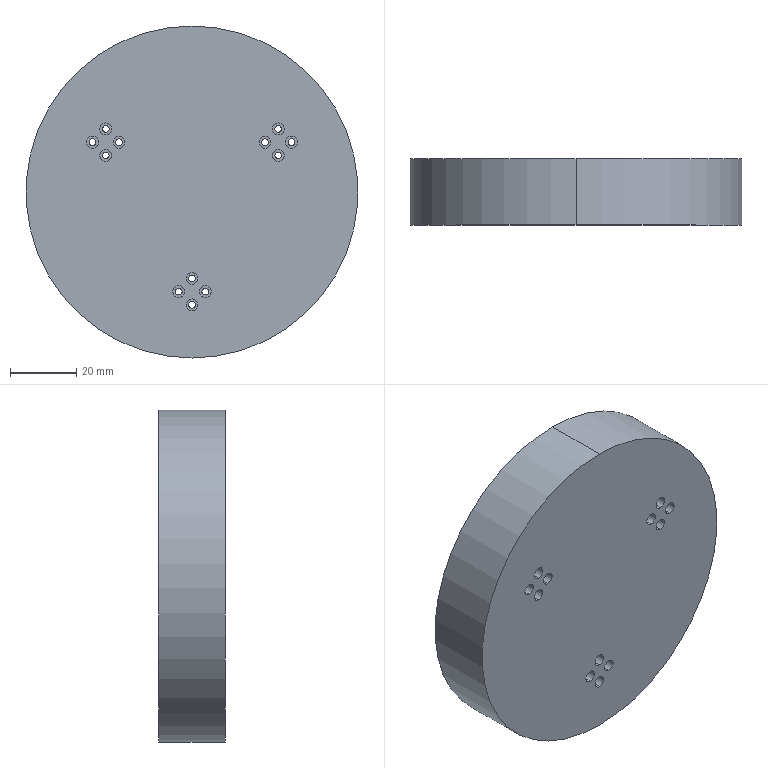Part | SolidWorks | features ICE 2, Cut 1, Extrusion 1 | 1 solid | 73 faces | box 100 x 20 x 100 mm | volume 148601 mm3 | cylinder 56 | plane 17 | commonest cylinder face diameters 2 x24 3.6 x24 15 x6 100 x2